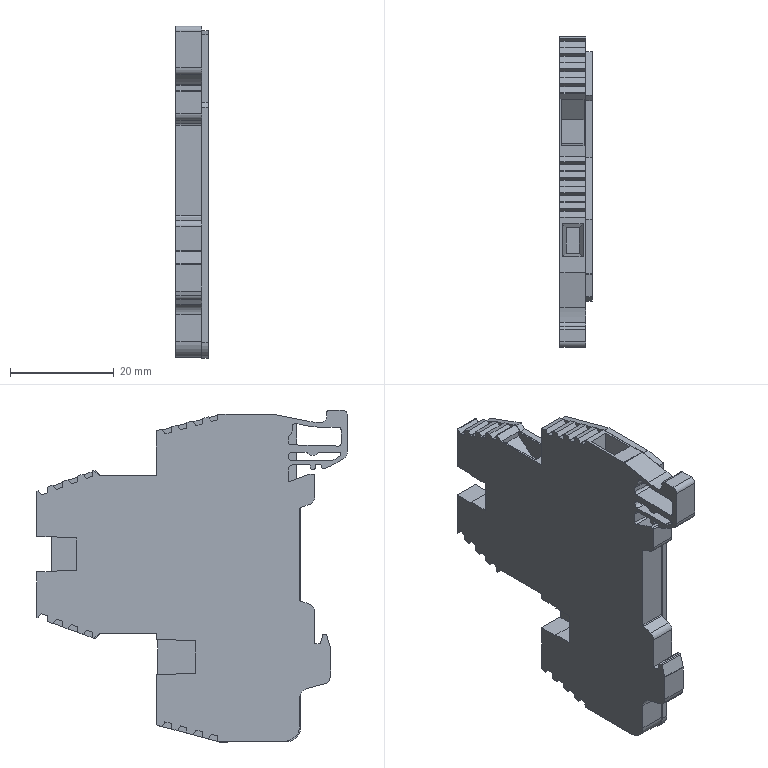Part | SolidWorks | 2 solids | 260 faces | box 6.25 x 60 x 64.152 mm | volume 14252 mm3 | plane 215 | cylinder 45 | commonest cylinder face diameters 1 x9 3.75 x7 0.6 x6 0.4 x3 2 x3 1.2 x2